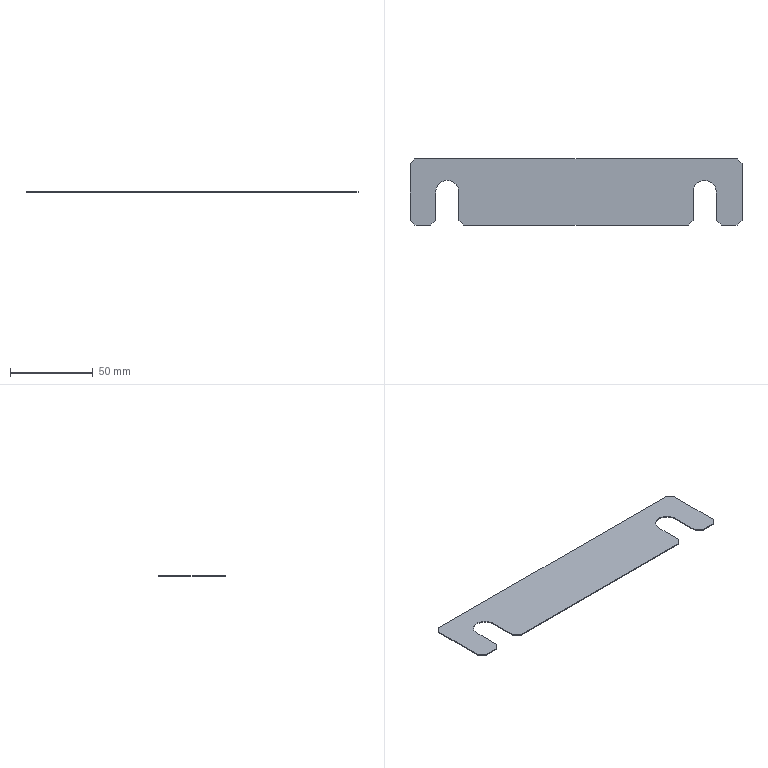Part | STEP file | J452-EBZ05-05-00 | 1 solid | 23 faces | box 200 x 40 x 0.5 mm | volume 3625 mm3 | plane 20 | cylinder 3 | commonest cylinder face diameters 14 x3